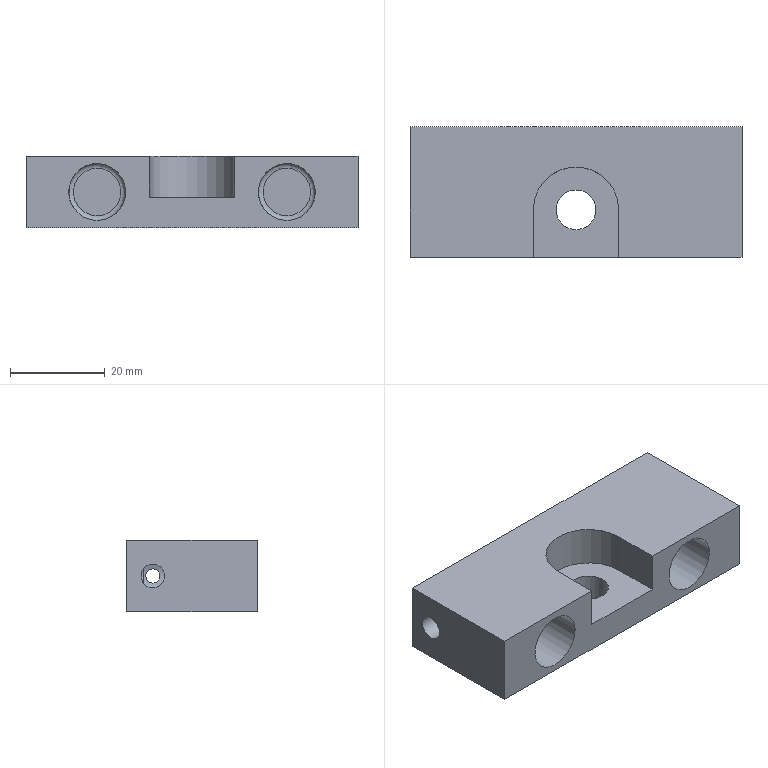NC program | NX | posted with a generic post | part box 70 x 27.5 x 15 mm
Lines 1 to 27 of 3781:
N10 G17 G21 G94 G90
(DRILLING_4 , TOOL : 点孔D10-150-90度)
N12 T01 M6
N14 G54
N16 G17 G0 G90 X-20. Y0. B0. C0. S1200 M3
N18 G43 Z20. H1
N20 G94 G81 G99 Z-1.5 B-180. C-180. F100. R3.
N22 X20.
N24 G80
N26 G0 X20. Y0. Z20.
N28 M5
(DRILLING_5 , TOOL : 钻头D11.5-106-143)
N30 T02 M6
N32 G54
N34 G17 G0 G90 X-20. Y0. B0. C0. S600 M3
N36 G43 Z20. H2
N38 G94 G83 G99 Z-24.8 B-180. C-180. F80. Q1.5 R3.
N40 X20.
N42 G80
N44 G0 X20. Y0. Z20.
N46 M5